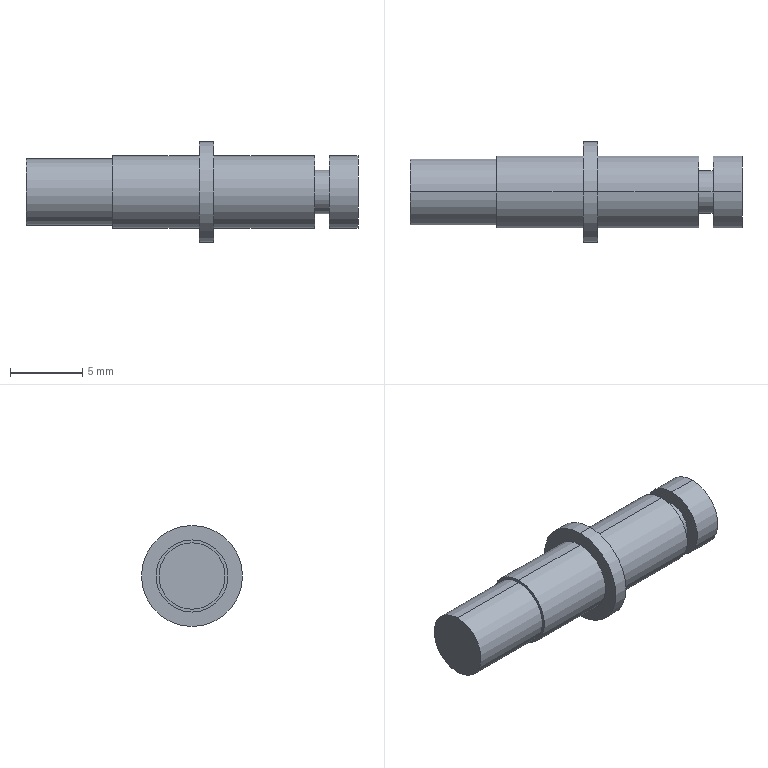Part | SolidWorks | features ICE 4, Revolution 2, Attribute 1, Extrusion 1, RevCut 1 | 1 solid | 19 faces | box 23 x 7 x 7 mm | volume 439.791 mm3 | cylinder 12 | plane 7 | commonest cylinder face diameters 5 x6 3 x2 4.6 x2 7 x2
STEP:
#1=CARTESIAN_POINT('',(10.,0.,-2.5));
#2=VERTEX_POINT('',#1);
#3=CARTESIAN_POINT('',(10.,0.,2.5));
#4=VERTEX_POINT('',#3);
#5=CARTESIAN_POINT('',(10.,0.,0.));
#6=DIRECTION('',(1.,0.,0.));
#7=DIRECTION('',(0.,0.,1.));
#8=AXIS2_PLACEMENT_3D('',#5,#6,#7);
#9=CIRCLE('',#8,2.5);
#10=EDGE_CURVE('',#2,#4,#9,.T.);
#11=ORIENTED_EDGE('',*,*,#10,.F.);
#12=CARTESIAN_POINT('',(4.,0.,-2.5));
#13=VERTEX_POINT('',#12);
#14=CARTESIAN_POINT('',(20.,0.,-2.5));
#15=DIRECTION('',(-1.,0.,0.));
#16=VECTOR('',#15,1000.);
#17=LINE('',#14,#16);
#18=EDGE_CURVE('',#2,#13,#17,.T.);
#19=ORIENTED_EDGE('',*,*,#18,.T.);
#20=CARTESIAN_POINT('',(4.,0.,2.5));
#21=VERTEX_POINT('',#20);
#22=CARTESIAN_POINT('',(4.,0.,0.));
#23=DIRECTION('',(-1.,0.,0.));
#24=DIRECTION('',(0.,0.,1.));
#25=AXIS2_PLACEMENT_3D('',#22,#23,#24);
#26=CIRCLE('',#25,2.5);
#27=EDGE_CURVE('',#21,#13,#26,.T.);
#28=ORIENTED_EDGE('',*,*,#27,.F.);
#29=CARTESIAN_POINT('',(20.,0.,2.5));
#30=DIRECTION('',(-1.,0.,0.));
#31=VECTOR('',#30,1000.);
#32=LINE('',#29,#31);
#33=EDGE_CURVE('',#4,#21,#32,.T.);
#34=ORIENTED_EDGE('',*,*,#33,.F.);
#35=EDGE_LOOP('',(#11,#19,#28,#34));
#36=FACE_OUTER_BOUND('',#35,.T.);
#37=CARTESIAN_POINT('',(20.,0.,0.));
#38=DIRECTION('',(-1.,0.,0.));
#39=DIRECTION('',(0.,0.,1.));
#40=AXIS2_PLACEMENT_3D('',#37,#38,#39);
#41=CYLINDRICAL_SURFACE('',#40,2.5);
#42=ADVANCED_FACE('',(#36),#41,.T.);
#43=CARTESIAN_POINT('',(4.,0.,2.3));
#44=VERTEX_POINT('',#43);
#45=CARTESIAN_POINT('',(4.,0.,-2.3));
#46=VERTEX_POINT('',#45);
#47=CARTESIAN_POINT('',(4.,0.,0.));
#48=DIRECTION('',(-1.,0.,0.));
#49=DIRECTION('',(0.,0.,1.));
#50=AXIS2_PLACEMENT_3D('',#47,#48,#49);
#51=CIRCLE('',#50,2.3);
#52=EDGE_CURVE('',#44,#46,#51,.T.);
#53=ORIENTED_EDGE('',*,*,#52,.T.);
#54=CARTESIAN_POINT('',(-2.,0.,-2.3));
#55=VERTEX_POINT('',#54);
#56=CARTESIAN_POINT('',(20.,0.,-2.3));
#57=DIRECTION('',(-1.,0.,0.));
#58=VECTOR('',#57,1000.);
#59=LINE('',#56,#58);
#60=EDGE_CURVE('',#46,#55,#59,.T.);
#61=ORIENTED_EDGE('',*,*,#60,.T.);
#62=CARTESIAN_POINT('',(-2.,0.,2.3));
#63=VERTEX_POINT('',#62);
#64=CARTESIAN_POINT('',(-2.,0.,0.));
#65=DIRECTION('',(-1.,0.,0.));
#66=DIRECTION('',(0.,0.,1.));
#67=AXIS2_PLACEMENT_3D('',#64,#65,#66);
#68=CIRCLE('',#67,2.3);
#69=EDGE_CURVE('',#63,#55,#68,.T.);
#70=ORIENTED_EDGE('',*,*,#69,.F.);
#71=CARTESIAN_POINT('',(20.,0.,2.3));
#72=DIRECTION('',(-1.,0.,0.));
#73=VECTOR('',#72,1000.);
#74=LINE('',#71,#73);
#75=EDGE_CURVE('',#44,#63,#74,.T.);
#76=ORIENTED_EDGE('',*,*,#75,.F.);
#77=EDGE_LOOP('',(#53,#61,#70,#76));
#78=FACE_OUTER_BOUND('',#77,.T.);
#79=CARTESIAN_POINT('',(20.,0.,0.));
#80=DIRECTION('',(-1.,0.,0.));
#81=DIRECTION('',(0.,0.,1.));
#82=AXIS2_PLACEMENT_3D('',#79,#80,#81);
#83=CYLINDRICAL_SURFACE('',#82,2.3);
#84=ADVANCED_FACE('',(#78),#83,.T.);
#85=CARTESIAN_POINT('',(10.,0.,-3.5));
#86=VERTEX_POINT('',#85);
#87=CARTESIAN_POINT('',(10.,0.,3.5));
#88=VERTEX_POINT('',#87);
#89=CARTESIAN_POINT('',(10.,0.,0.));
#90=DIRECTION('',(1.,0.,0.));
#91=DIRECTION('',(0.,0.,-1.));
#92=AXIS2_PLACEMENT_3D('',#89,#90,#91);
#93=CIRCLE('',#92,3.5);
#94=EDGE_CURVE('',#86,#88,#93,.T.);
#95=ORIENTED_EDGE('',*,*,#94,.T.);
#96=CARTESIAN_POINT('',(11.,0.,3.5));
#97=VERTEX_POINT('',#96);
#98=CARTESIAN_POINT('',(20.,0.,3.5));
#99=DIRECTION('',(1.,0.,0.));
#100=VECTOR('',#99,1000.);
#101=LINE('',#98,#100);
#102=EDGE_CURVE('',#88,#97,#101,.T.);
#103=ORIENTED_EDGE('',*,*,#102,.T.);
#104=CARTESIAN_POINT('',(11.,0.,-3.5));
#105=VERTEX_POINT('',#104);
#106=CARTESIAN_POINT('',(11.,0.,0.));
#107=DIRECTION('',(1.,0.,0.));
#108=DIRECTION('',(0.,0.,-1.));
#109=AXIS2_PLACEMENT_3D('',#106,#107,#108);
#110=CIRCLE('',#109,3.5);
#111=EDGE_CURVE('',#105,#97,#110,.T.);
#112=ORIENTED_EDGE('',*,*,#111,.F.);
#113=CARTESIAN_POINT('',(20.,0.,-3.5));
#114=DIRECTION('',(1.,0.,0.));
#115=VECTOR('',#114,1000.);
#116=LINE('',#113,#115);
#117=EDGE_CURVE('',#86,#105,#116,.T.);
#118=ORIENTED_EDGE('',*,*,#117,.F.);
#119=EDGE_LOOP('',(#95,#103,#112,#118));
#120=FACE_OUTER_BOUND('',#119,.T.);
#121=CARTESIAN_POINT('',(20.,0.,0.));
#122=DIRECTION('',(1.,0.,0.));
#123=DIRECTION('',(0.,0.,-1.));
#124=AXIS2_PLACEMENT_3D('',#121,#122,#123);
#125=CYLINDRICAL_SURFACE('',#124,3.5);
#126=ADVANCED_FACE('',(#120),#125,.T.);
#127=CARTESIAN_POINT('',(21.,0.,-2.5));
#128=VERTEX_POINT('',#127);
#129=CARTESIAN_POINT('',(21.,0.,2.5));
#130=VERTEX_POINT('',#129);
#131=CARTESIAN_POINT('',(21.,0.,0.));
#132=DIRECTION('',(1.,0.,0.));
#133=DIRECTION('',(0.,0.,-1.));
#134=AXIS2_PLACEMENT_3D('',#131,#132,#133);
#135=CIRCLE('',#134,2.5);
#136=EDGE_CURVE('',#128,#130,#135,.T.);
#137=ORIENTED_EDGE('',*,*,#136,.F.);
#138=CARTESIAN_POINT('',(18.994,0.,-2.5));
#139=VERTEX_POINT('',#138);
#140=CARTESIAN_POINT('',(20.,0.,-2.5));
#141=DIRECTION('',(-1.,0.,0.));
#142=VECTOR('',#141,1000.);
#143=LINE('',#140,#142);
#144=EDGE_CURVE('',#128,#139,#143,.T.);
#145=ORIENTED_EDGE('',*,*,#144,.T.);
#146=CARTESIAN_POINT('',(18.994,0.,2.5));
#147=VERTEX_POINT('',#146);
#148=CARTESIAN_POINT('',(18.994,0.,0.));
#149=DIRECTION('',(1.,0.,0.));
#150=DIRECTION('',(0.,0.,-1.));
#151=AXIS2_PLACEMENT_3D('',#148,#149,#150);
#152=CIRCLE('',#151,2.5);
#153=EDGE_CURVE('',#139,#147,#152,.T.);
#154=ORIENTED_EDGE('',*,*,#153,.T.);
#155=CARTESIAN_POINT('',(20.,0.,2.5));
#156=DIRECTION('',(-1.,0.,0.));
#157=VECTOR('',#156,1000.);
#158=LINE('',#155,#157);
#159=EDGE_CURVE('',#130,#147,#158,.T.);
#160=ORIENTED_EDGE('',*,*,#159,.F.);
#161=EDGE_LOOP('',(#137,#145,#154,#160));
#162=FACE_OUTER_BOUND('',#161,.T.);
#163=CARTESIAN_POINT('',(20.,0.,0.));
#164=DIRECTION('',(-1.,0.,0.));
#165=DIRECTION('',(0.,0.,1.));
#166=AXIS2_PLACEMENT_3D('',#163,#164,#165);
#167=CYLINDRICAL_SURFACE('',#166,2.5);
#168=ADVANCED_FACE('',(#162),#167,.T.);
#169=CARTESIAN_POINT('',(17.994,0.,-1.5));
#170=VERTEX_POINT('',#169);
#171=CARTESIAN_POINT('',(17.994,0.,1.5));
#172=VERTEX_POINT('',#171);
#173=CARTESIAN_POINT('',(17.994,0.,0.));
#174=DIRECTION('',(1.,0.,0.));
#175=DIRECTION('',(0.,0.,-1.));
#176=AXIS2_PLACEMENT_3D('',#173,#174,#175);
#177=CIRCLE('',#176,1.5);
#178=EDGE_CURVE('',#170,#172,#177,.T.);
#179=ORIENTED_EDGE('',*,*,#178,.T.);
#180=CARTESIAN_POINT('',(18.994,0.,1.5));
#181=VERTEX_POINT('',#180);
#182=CARTESIAN_POINT('',(20.994,0.,1.5));
#183=DIRECTION('',(1.,0.,0.));
#184=VECTOR('',#183,1000.);
#185=LINE('',#182,#184);
#186=EDGE_CURVE('',#172,#181,#185,.T.);
#187=ORIENTED_EDGE('',*,*,#186,.T.);
#188=CARTESIAN_POINT('',(18.994,0.,-1.5));
#189=VERTEX_POINT('',#188);
#190=CARTESIAN_POINT('',(18.994,0.,0.));
#191=DIRECTION('',(1.,0.,0.));
#192=DIRECTION('',(0.,0.,-1.));
#193=AXIS2_PLACEMENT_3D('',#190,#191,#192);
#194=CIRCLE('',#193,1.5);
#195=EDGE_CURVE('',#189,#181,#194,.T.);
#196=ORIENTED_EDGE('',*,*,#195,.F.);
#197=CARTESIAN_POINT('',(20.994,0.,-1.5));
#198=DIRECTION('',(1.,0.,0.));
#199=VECTOR('',#198,1000.);
#200=LINE('',#197,#199);
#201=EDGE_CURVE('',#170,#189,#200,.T.);
#202=ORIENTED_EDGE('',*,*,#201,.F.);
#203=EDGE_LOOP('',(#179,#187,#196,#202));
#204=FACE_OUTER_BOUND('',#203,.T.);
#205=CARTESIAN_POINT('',(20.994,0.,0.));
#206=DIRECTION('',(1.,0.,0.));
#207=DIRECTION('',(0.,0.,-1.));
#208=AXIS2_PLACEMENT_3D('',#205,#206,#207);
#209=CYLINDRICAL_SURFACE('',#208,1.5);
#210=ADVANCED_FACE('',(#204),#209,.T.);
#211=CARTESIAN_POINT('',(17.994,0.,-2.5));
#212=VERTEX_POINT('',#211);
#213=CARTESIAN_POINT('',(17.994,0.,2.5));
#214=VERTEX_POINT('',#213);
#215=CARTESIAN_POINT('',(17.994,0.,0.));
#216=DIRECTION('',(1.,0.,0.));
#217=DIRECTION('',(0.,0.,-1.));
#218=AXIS2_PLACEMENT_3D('',#215,#216,#217);
#219=CIRCLE('',#218,2.5);
#220=EDGE_CURVE('',#212,#214,#219,.T.);
#221=ORIENTED_EDGE('',*,*,#220,.F.);
#222=CARTESIAN_POINT('',(11.,0.,-2.5));
#223=VERTEX_POINT('',#222);
#224=CARTESIAN_POINT('',(20.,0.,-2.5));
#225=DIRECTION('',(-1.,0.,0.));
#226=VECTOR('',#225,1000.);
#227=LINE('',#224,#226);
#228=EDGE_CURVE('',#212,#223,#227,.T.);
#229=ORIENTED_EDGE('',*,*,#228,.T.);
#230=CARTESIAN_POINT('',(11.,0.,2.5));
#231=VERTEX_POINT('',#230);
#232=CARTESIAN_POINT('',(11.,0.,0.));
#233=DIRECTION('',(-1.,0.,0.));
#234=DIRECTION('',(0.,0.,-1.));
#235=AXIS2_PLACEMENT_3D('',#232,#233,#234);
#236=CIRCLE('',#235,2.5);
#237=EDGE_CURVE('',#231,#223,#236,.T.);
#238=ORIENTED_EDGE('',*,*,#237,.F.);
#239=CARTESIAN_POINT('',(20.,0.,2.5));
#240=DIRECTION('',(-1.,0.,0.));
#241=VECTOR('',#240,1000.);
#242=LINE('',#239,#241);
#243=EDGE_CURVE('',#214,#231,#242,.T.);
#244=ORIENTED_EDGE('',*,*,#243,.F.);
#245=EDGE_LOOP('',(#221,#229,#238,#244));
#246=FACE_OUTER_BOUND('',#245,.T.);
#247=CARTESIAN_POINT('',(20.,0.,0.));
#248=DIRECTION('',(-1.,0.,0.));
#249=DIRECTION('',(0.,0.,1.));
#250=AXIS2_PLACEMENT_3D('',#247,#248,#249);
#251=CYLINDRICAL_SURFACE('',#250,2.5);
#252=ADVANCED_FACE('',(#246),#251,.T.);
#253=ORIENTED_EDGE('',*,*,#228,.F.);
#254=CARTESIAN_POINT('',(17.994,0.,0.));
#255=DIRECTION('',(1.,0.,0.));
#256=DIRECTION('',(0.,0.,-1.));
#257=AXIS2_PLACEMENT_3D('',#254,#255,#256);
#258=CIRCLE('',#257,2.5);
#259=EDGE_CURVE('',#214,#212,#258,.T.);
#260=ORIENTED_EDGE('',*,*,#259,.F.);
#261=ORIENTED_EDGE('',*,*,#243,.T.);
#262=CARTESIAN_POINT('',(11.,0.,0.));
#263=DIRECTION('',(-1.,0.,0.));
#264=DIRECTION('',(0.,0.,-1.));
#265=AXIS2_PLACEMENT_3D('',#262,#263,#264);
#266=CIRCLE('',#265,2.5);
#267=EDGE_CURVE('',#223,#231,#266,.T.);
#268=ORIENTED_EDGE('',*,*,#267,.F.);
#269=EDGE_LOOP('',(#253,#260,#261,#268));
#270=FACE_OUTER_BOUND('',#269,.T.);
#271=CARTESIAN_POINT('',(20.,0.,0.));
#272=DIRECTION('',(-1.,0.,0.));
#273=DIRECTION('',(0.,0.,1.));
#274=AXIS2_PLACEMENT_3D('',#271,#272,#273);
#275=CYLINDRICAL_SURFACE('',#274,2.5);
#276=ADVANCED_FACE('',(#270),#275,.T.);
#277=CARTESIAN_POINT('',(18.994,0.,0.));
#278=DIRECTION('',(1.,0.,0.));
#279=DIRECTION('',(0.,0.,-1.));
#280=AXIS2_PLACEMENT_3D('',#277,#278,#279);
#281=CIRCLE('',#280,2.5);
#282=EDGE_CURVE('',#147,#139,#281,.T.);
#283=ORIENTED_EDGE('',*,*,#282,.F.);
#284=ORIENTED_EDGE('',*,*,#153,.F.);
#285=EDGE_LOOP('',(#283,#284));
#286=FACE_OUTER_BOUND('',#285,.T.);
#287=ORIENTED_EDGE('',*,*,#195,.T.);
#288=CARTESIAN_POINT('',(18.994,0.,0.));
#289=DIRECTION('',(1.,0.,0.));
#290=DIRECTION('',(0.,0.,-1.));
#291=AXIS2_PLACEMENT_3D('',#288,#289,#290);
#292=CIRCLE('',#291,1.5);
#293=EDGE_CURVE('',#181,#189,#292,.T.);
#294=ORIENTED_EDGE('',*,*,#293,.T.);
#295=EDGE_LOOP('',(#287,#294));
#296=FACE_BOUND('',#295,.T.);
#297=CARTESIAN_POINT('',(18.994,2.5,0.));
#298=DIRECTION('',(1.,0.,0.));
#299=DIRECTION('',(0.,0.,-1.));
#300=AXIS2_PLACEMENT_3D('',#297,#298,#299);
#301=PLANE('',#300);
#302=ADVANCED_FACE('',(#286,#296),#301,.F.);
#303=ORIENTED_EDGE('',*,*,#186,.F.);
#304=CARTESIAN_POINT('',(17.994,0.,0.));
#305=DIRECTION('',(1.,0.,0.));
#306=DIRECTION('',(0.,0.,-1.));
#307=AXIS2_PLACEMENT_3D('',#304,#305,#306);
#308=CIRCLE('',#307,1.5);
#309=EDGE_CURVE('',#172,#170,#308,.T.);
#310=ORIENTED_EDGE('',*,*,#309,.T.);
#311=ORIENTED_EDGE('',*,*,#201,.T.);
#312=ORIENTED_EDGE('',*,*,#293,.F.);
#313=EDGE_LOOP('',(#303,#310,#311,#312));
#314=FACE_OUTER_BOUND('',#313,.T.);
#315=CARTESIAN_POINT('',(20.994,0.,0.));
#316=DIRECTION('',(1.,0.,0.));
#317=DIRECTION('',(0.,0.,-1.));
#318=AXIS2_PLACEMENT_3D('',#315,#316,#317);
#319=CYLINDRICAL_SURFACE('',#318,1.5);
#320=ADVANCED_FACE('',(#314),#319,.T.);
#321=ORIENTED_EDGE('',*,*,#178,.F.);
#322=ORIENTED_EDGE('',*,*,#309,.F.);
#323=EDGE_LOOP('',(#321,#322));
#324=FACE_BOUND('',#323,.T.);
#325=ORIENTED_EDGE('',*,*,#259,.T.);
#326=ORIENTED_EDGE('',*,*,#220,.T.);
#327=EDGE_LOOP('',(#325,#326));
#328=FACE_OUTER_BOUND('',#327,.T.);
#329=CARTESIAN_POINT('',(17.994,1.5,0.));
#330=DIRECTION('',(-1.,0.,0.));
#331=DIRECTION('',(0.,0.,1.));
#332=AXIS2_PLACEMENT_3D('',#329,#330,#331);
#333=PLANE('',#332);
#334=ADVANCED_FACE('',(#324,#328),#333,.F.);
#335=ORIENTED_EDGE('',*,*,#144,.F.);
#336=CARTESIAN_POINT('',(21.,0.,0.));
#337=DIRECTION('',(1.,0.,0.));
#338=DIRECTION('',(0.,0.,-1.));
#339=AXIS2_PLACEMENT_3D('',#336,#337,#338);
#340=CIRCLE('',#339,2.5);
#341=EDGE_CURVE('',#130,#128,#340,.T.);
#342=ORIENTED_EDGE('',*,*,#341,.F.);
#343=ORIENTED_EDGE('',*,*,#159,.T.);
#344=ORIENTED_EDGE('',*,*,#282,.T.);
#345=EDGE_LOOP('',(#335,#342,#343,#344));
#346=FACE_OUTER_BOUND('',#345,.T.);
#347=CARTESIAN_POINT('',(20.,0.,0.));
#348=DIRECTION('',(-1.,0.,0.));
#349=DIRECTION('',(0.,0.,1.));
#350=AXIS2_PLACEMENT_3D('',#347,#348,#349);
#351=CYLINDRICAL_SURFACE('',#350,2.5);
#352=ADVANCED_FACE('',(#346),#351,.T.);
#353=CARTESIAN_POINT('',(10.,0.,0.));
#354=DIRECTION('',(1.,0.,0.));
#355=DIRECTION('',(0.,0.,1.));
#356=AXIS2_PLACEMENT_3D('',#353,#354,#355);
#357=CIRCLE('',#356,2.5);
#358=EDGE_CURVE('',#4,#2,#357,.T.);
#359=ORIENTED_EDGE('',*,*,#358,.T.);
#360=ORIENTED_EDGE('',*,*,#10,.T.);
#361=EDGE_LOOP('',(#359,#360));
#362=FACE_BOUND('',#361,.T.);
#363=ORIENTED_EDGE('',*,*,#94,.F.);
#364=CARTESIAN_POINT('',(10.,0.,0.));
#365=DIRECTION('',(1.,0.,0.));
#366=DIRECTION('',(0.,0.,-1.));
#367=AXIS2_PLACEMENT_3D('',#364,#365,#366);
#368=CIRCLE('',#367,3.5);
#369=EDGE_CURVE('',#88,#86,#368,.T.);
#370=ORIENTED_EDGE('',*,*,#369,.F.);
#371=EDGE_LOOP('',(#363,#370));
#372=FACE_OUTER_BOUND('',#371,.T.);
#373=CARTESIAN_POINT('',(10.,2.5,0.));
#374=DIRECTION('',(-1.,0.,0.));
#375=DIRECTION('',(0.,0.,1.));
#376=AXIS2_PLACEMENT_3D('',#373,#374,#375);
#377=PLANE('',#376);
#378=ADVANCED_FACE('',(#362,#372),#377,.T.);
#379=ORIENTED_EDGE('',*,*,#102,.F.);
#380=ORIENTED_EDGE('',*,*,#369,.T.);
#381=ORIENTED_EDGE('',*,*,#117,.T.);
#382=CARTESIAN_POINT('',(11.,0.,0.));
#383=DIRECTION('',(1.,0.,0.));
#384=DIRECTION('',(0.,0.,-1.));
#385=AXIS2_PLACEMENT_3D('',#382,#383,#384);
#386=CIRCLE('',#385,3.5);
#387=EDGE_CURVE('',#97,#105,#386,.T.);
#388=ORIENTED_EDGE('',*,*,#387,.F.);
#389=EDGE_LOOP('',(#379,#380,#381,#388));
#390=FACE_OUTER_BOUND('',#389,.T.);
#391=CARTESIAN_POINT('',(20.,0.,0.));
#392=DIRECTION('',(1.,0.,0.));
#393=DIRECTION('',(0.,0.,-1.));
#394=AXIS2_PLACEMENT_3D('',#391,#392,#393);
#395=CYLINDRICAL_SURFACE('',#394,3.5);
#396=ADVANCED_FACE('',(#390),#395,.T.);
#397=ORIENTED_EDGE('',*,*,#111,.T.);
#398=ORIENTED_EDGE('',*,*,#387,.T.);
#399=EDGE_LOOP('',(#397,#398));
#400=FACE_OUTER_BOUND('',#399,.T.);
#401=ORIENTED_EDGE('',*,*,#237,.T.);
#402=ORIENTED_EDGE('',*,*,#267,.T.);
#403=EDGE_LOOP('',(#401,#402));
#404=FACE_BOUND('',#403,.T.);
#405=CARTESIAN_POINT('',(11.,2.5,0.));
#406=DIRECTION('',(1.,0.,0.));
#407=DIRECTION('',(0.,0.,-1.));
#408=AXIS2_PLACEMENT_3D('',#405,#406,#407);
#409=PLANE('',#408);
#410=ADVANCED_FACE('',(#400,#404),#409,.T.);
#411=ORIENTED_EDGE('',*,*,#69,.T.);
#412=CARTESIAN_POINT('',(-2.,0.,0.));
#413=DIRECTION('',(-1.,0.,0.));
#414=DIRECTION('',(0.,0.,1.));
#415=AXIS2_PLACEMENT_3D('',#412,#413,#414);
#416=CIRCLE('',#415,2.3);
#417=EDGE_CURVE('',#55,#63,#416,.T.);
#418=ORIENTED_EDGE('',*,*,#417,.T.);
#419=EDGE_LOOP('',(#411,#418));
#420=FACE_OUTER_BOUND('',#419,.T.);
#421=CARTESIAN_POINT('',(-2.,0.,0.));
#422=DIRECTION('',(-1.,0.,0.));
#423=DIRECTION('',(0.,0.,1.));
#424=AXIS2_PLACEMENT_3D('',#421,#422,#423);
#425=PLANE('',#424);
#426=ADVANCED_FACE('',(#420),#425,.T.);
#427=ORIENTED_EDGE('',*,*,#60,.F.);
#428=CARTESIAN_POINT('',(4.,0.,0.));
#429=DIRECTION('',(-1.,0.,0.));
#430=DIRECTION('',(0.,0.,1.));
#431=AXIS2_PLACEMENT_3D('',#428,#429,#430);
#432=CIRCLE('',#431,2.3);
#433=EDGE_CURVE('',#46,#44,#432,.T.);
#434=ORIENTED_EDGE('',*,*,#433,.T.);
#435=ORIENTED_EDGE('',*,*,#75,.T.);
#436=ORIENTED_EDGE('',*,*,#417,.F.);
#437=EDGE_LOOP('',(#427,#434,#435,#436));
#438=FACE_OUTER_BOUND('',#437,.T.);
#439=CARTESIAN_POINT('',(20.,0.,0.));
#440=DIRECTION('',(-1.,0.,0.));
#441=DIRECTION('',(0.,0.,1.));
#442=AXIS2_PLACEMENT_3D('',#439,#440,#441);
#443=CYLINDRICAL_SURFACE('',#442,2.3);
#444=ADVANCED_FACE('',(#438),#443,.T.);
#445=ORIENTED_EDGE('',*,*,#52,.F.);
#446=ORIENTED_EDGE('',*,*,#433,.F.);
#447=EDGE_LOOP('',(#445,#446));
#448=FACE_BOUND('',#447,.T.);
#449=ORIENTED_EDGE('',*,*,#27,.T.);
#450=CARTESIAN_POINT('',(4.,0.,0.));
#451=DIRECTION('',(-1.,0.,0.));
#452=DIRECTION('',(0.,0.,1.));
#453=AXIS2_PLACEMENT_3D('',#450,#451,#452);
#454=CIRCLE('',#453,2.5);
#455=EDGE_CURVE('',#13,#21,#454,.T.);
#456=ORIENTED_EDGE('',*,*,#455,.T.);
#457=EDGE_LOOP('',(#449,#456));
#458=FACE_OUTER_BOUND('',#457,.T.);
#459=CARTESIAN_POINT('',(4.,0.,0.));
#460=DIRECTION('',(-1.,0.,0.));
#461=DIRECTION('',(0.,0.,1.));
#462=AXIS2_PLACEMENT_3D('',#459,#460,#461);
#463=PLANE('',#462);
#464=ADVANCED_FACE('',(#448,#458),#463,.T.);
#465=ORIENTED_EDGE('',*,*,#18,.F.);
#466=ORIENTED_EDGE('',*,*,#358,.F.);
#467=ORIENTED_EDGE('',*,*,#33,.T.);
#468=ORIENTED_EDGE('',*,*,#455,.F.);
#469=EDGE_LOOP('',(#465,#466,#467,#468));
#470=FACE_OUTER_BOUND('',#469,.T.);
#471=CARTESIAN_POINT('',(20.,0.,0.));
#472=DIRECTION('',(-1.,0.,0.));
#473=DIRECTION('',(0.,0.,1.));
#474=AXIS2_PLACEMENT_3D('',#471,#472,#473);
#475=CYLINDRICAL_SURFACE('',#474,2.5);
#476=ADVANCED_FACE('',(#470),#475,.T.);
#477=ORIENTED_EDGE('',*,*,#341,.T.);
#478=ORIENTED_EDGE('',*,*,#136,.T.);
#479=EDGE_LOOP('',(#477,#478));
#480=FACE_OUTER_BOUND('',#479,.T.);
#481=CARTESIAN_POINT('',(21.,0.,0.));
#482=DIRECTION('',(1.,0.,0.));
#483=DIRECTION('',(0.,0.,-1.));
#484=AXIS2_PLACEMENT_3D('',#481,#482,#483);
#485=PLANE('',#484);
#486=ADVANCED_FACE('',(#480),#485,.T.);
#487=CLOSED_SHELL('',(#42,#84,#126,#168,#210,#252,#276,#302,#320,#334,#352,#378,#396,#410,#426,#444,#464,#476,#486));
#488=MANIFOLD_SOLID_BREP('',#487);
#489=CARTESIAN_POINT('',(0.,0.,0.));
#490=DIRECTION('',(0.,0.,1.));
#491=DIRECTION('',(1.,0.,0.));
#492=AXIS2_PLACEMENT_3D('',#489,#490,#491);
#493=(LENGTH_UNIT()NAMED_UNIT(*)SI_UNIT(.MILLI.,.METRE.));
#494=UNCERTAINTY_MEASURE_WITH_UNIT(LENGTH_MEASURE(0.00001),#493,'','');
#495=(NAMED_UNIT(*)PLANE_ANGLE_UNIT()SI_UNIT($,.RADIAN.));
#496=(NAMED_UNIT(*)SI_UNIT($,.STERADIAN.)SOLID_ANGLE_UNIT());
#497=(GEOMETRIC_REPRESENTATION_CONTEXT(3)GLOBAL_UNCERTAINTY_ASSIGNED_CONTEXT((#494))GLOBAL_UNIT_ASSIGNED_CONTEXT((#493,#495,#496))REPRESENTATION_CONTEXT('',''));
#498=ADVANCED_BREP_SHAPE_REPRESENTATION('',(#488,#492),#497);